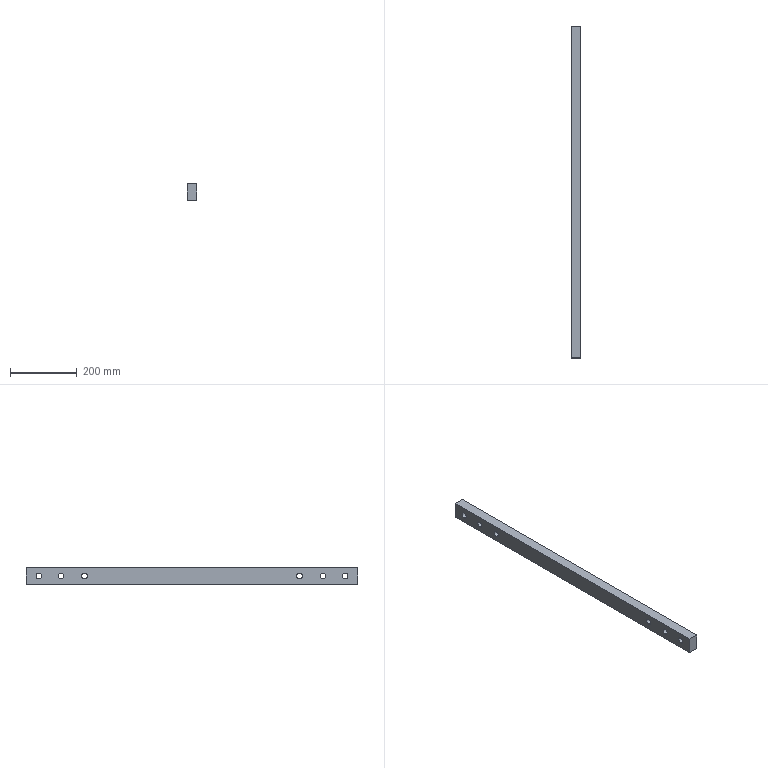Part | SolidWorks | features BaseBody 1 | 1 solid | 18 faces | box 30 x 998 x 50 mm | volume 1456144 mm3 | cylinder 12 | plane 6 | commonest cylinder face diameters 17 x12
STEP:
#1=CARTESIAN_POINT('',(15.,38.5,-8.5));
#2=VERTEX_POINT('',#1);
#3=CARTESIAN_POINT('',(15.,38.5,8.5));
#4=VERTEX_POINT('',#3);
#5=CARTESIAN_POINT('',(15.,38.5,0.));
#6=DIRECTION('',(-1.,0.,0.));
#7=DIRECTION('',(0.,0.,1.));
#8=AXIS2_PLACEMENT_3D('',#5,#6,#7);
#9=CIRCLE('',#8,8.5);
#10=EDGE_CURVE('',#2,#4,#9,.T.);
#11=ORIENTED_EDGE('',*,*,#10,.F.);
#12=CARTESIAN_POINT('',(-15.,38.5,-8.5));
#13=VERTEX_POINT('',#12);
#14=CARTESIAN_POINT('',(15.,38.5,-8.5));
#15=DIRECTION('',(-1.,0.,0.));
#16=VECTOR('',#15,1000.);
#17=LINE('',#14,#16);
#18=EDGE_CURVE('',#2,#13,#17,.T.);
#19=ORIENTED_EDGE('',*,*,#18,.T.);
#20=CARTESIAN_POINT('',(-15.,38.5,8.5));
#21=VERTEX_POINT('',#20);
#22=CARTESIAN_POINT('',(-15.,38.5,0.));
#23=DIRECTION('',(-1.,0.,0.));
#24=DIRECTION('',(0.,0.,1.));
#25=AXIS2_PLACEMENT_3D('',#22,#23,#24);
#26=CIRCLE('',#25,8.5);
#27=EDGE_CURVE('',#13,#21,#26,.T.);
#28=ORIENTED_EDGE('',*,*,#27,.T.);
#29=CARTESIAN_POINT('',(15.,38.5,8.5));
#30=DIRECTION('',(-1.,0.,0.));
#31=VECTOR('',#30,1000.);
#32=LINE('',#29,#31);
#33=EDGE_CURVE('',#4,#21,#32,.T.);
#34=ORIENTED_EDGE('',*,*,#33,.F.);
#35=EDGE_LOOP('',(#11,#19,#28,#34));
#36=FACE_OUTER_BOUND('',#35,.T.);
#37=CARTESIAN_POINT('',(15.,38.5,0.));
#38=DIRECTION('',(-1.,0.,0.));
#39=DIRECTION('',(0.,0.,1.));
#40=AXIS2_PLACEMENT_3D('',#37,#38,#39);
#41=CYLINDRICAL_SURFACE('',#40,8.5);
#42=ADVANCED_FACE('',(#36),#41,.F.);
#43=CARTESIAN_POINT('',(15.,822.359,-8.5));
#44=VERTEX_POINT('',#43);
#45=CARTESIAN_POINT('',(15.,822.359,8.5));
#46=VERTEX_POINT('',#45);
#47=CARTESIAN_POINT('',(15.,822.359,0.));
#48=DIRECTION('',(-1.,0.,0.));
#49=DIRECTION('',(0.,0.,-1.));
#50=AXIS2_PLACEMENT_3D('',#47,#48,#49);
#51=CIRCLE('',#50,8.5);
#52=EDGE_CURVE('',#44,#46,#51,.T.);
#53=ORIENTED_EDGE('',*,*,#52,.F.);
#54=CARTESIAN_POINT('',(-15.,822.359,-8.5));
#55=VERTEX_POINT('',#54);
#56=CARTESIAN_POINT('',(15.,822.359,-8.5));
#57=DIRECTION('',(-1.,0.,0.));
#58=VECTOR('',#57,1000.);
#59=LINE('',#56,#58);
#60=EDGE_CURVE('',#44,#55,#59,.T.);
#61=ORIENTED_EDGE('',*,*,#60,.T.);
#62=CARTESIAN_POINT('',(-15.,822.359,8.5));
#63=VERTEX_POINT('',#62);
#64=CARTESIAN_POINT('',(-15.,822.359,0.));
#65=DIRECTION('',(-1.,0.,0.));
#66=DIRECTION('',(0.,0.,-1.));
#67=AXIS2_PLACEMENT_3D('',#64,#65,#66);
#68=CIRCLE('',#67,8.5);
#69=EDGE_CURVE('',#55,#63,#68,.T.);
#70=ORIENTED_EDGE('',*,*,#69,.T.);
#71=CARTESIAN_POINT('',(15.,822.359,8.5));
#72=DIRECTION('',(-1.,0.,0.));
#73=VECTOR('',#72,1000.);
#74=LINE('',#71,#73);
#75=EDGE_CURVE('',#46,#63,#74,.T.);
#76=ORIENTED_EDGE('',*,*,#75,.F.);
#77=EDGE_LOOP('',(#53,#61,#70,#76));
#78=FACE_OUTER_BOUND('',#77,.T.);
#79=CARTESIAN_POINT('',(15.,822.359,0.));
#80=DIRECTION('',(-1.,0.,0.));
#81=DIRECTION('',(0.,0.,1.));
#82=AXIS2_PLACEMENT_3D('',#79,#80,#81);
#83=CYLINDRICAL_SURFACE('',#82,8.5);
#84=ADVANCED_FACE('',(#78),#83,.F.);
#85=CARTESIAN_POINT('',(15.,175.641,-8.5));
#86=VERTEX_POINT('',#85);
#87=CARTESIAN_POINT('',(15.,175.641,8.5));
#88=VERTEX_POINT('',#87);
#89=CARTESIAN_POINT('',(15.,175.641,0.));
#90=DIRECTION('',(-1.,0.,0.));
#91=DIRECTION('',(0.,0.,1.));
#92=AXIS2_PLACEMENT_3D('',#89,#90,#91);
#93=CIRCLE('',#92,8.5);
#94=EDGE_CURVE('',#86,#88,#93,.T.);
#95=ORIENTED_EDGE('',*,*,#94,.F.);
#96=CARTESIAN_POINT('',(-15.,175.641,-8.5));
#97=VERTEX_POINT('',#96);
#98=CARTESIAN_POINT('',(15.,175.641,-8.5));
#99=DIRECTION('',(-1.,0.,0.));
#100=VECTOR('',#99,1000.);
#101=LINE('',#98,#100);
#102=EDGE_CURVE('',#86,#97,#101,.T.);
#103=ORIENTED_EDGE('',*,*,#102,.T.);
#104=CARTESIAN_POINT('',(-15.,175.641,8.5));
#105=VERTEX_POINT('',#104);
#106=CARTESIAN_POINT('',(-15.,175.641,0.));
#107=DIRECTION('',(-1.,0.,0.));
#108=DIRECTION('',(0.,0.,1.));
#109=AXIS2_PLACEMENT_3D('',#106,#107,#108);
#110=CIRCLE('',#109,8.5);
#111=EDGE_CURVE('',#97,#105,#110,.T.);
#112=ORIENTED_EDGE('',*,*,#111,.T.);
#113=CARTESIAN_POINT('',(15.,175.641,8.5));
#114=DIRECTION('',(-1.,0.,0.));
#115=VECTOR('',#114,1000.);
#116=LINE('',#113,#115);
#117=EDGE_CURVE('',#88,#105,#116,.T.);
#118=ORIENTED_EDGE('',*,*,#117,.F.);
#119=EDGE_LOOP('',(#95,#103,#112,#118));
#120=FACE_OUTER_BOUND('',#119,.T.);
#121=CARTESIAN_POINT('',(15.,175.641,0.));
#122=DIRECTION('',(-1.,0.,0.));
#123=DIRECTION('',(0.,0.,1.));
#124=AXIS2_PLACEMENT_3D('',#121,#122,#123);
#125=CYLINDRICAL_SURFACE('',#124,8.5);
#126=ADVANCED_FACE('',(#120),#125,.F.);
#127=CARTESIAN_POINT('',(15.,892.899,-8.5));
#128=VERTEX_POINT('',#127);
#129=CARTESIAN_POINT('',(15.,892.899,8.5));
#130=VERTEX_POINT('',#129);
#131=CARTESIAN_POINT('',(15.,892.899,0.));
#132=DIRECTION('',(-1.,0.,0.));
#133=DIRECTION('',(0.,0.,-1.));
#134=AXIS2_PLACEMENT_3D('',#131,#132,#133);
#135=CIRCLE('',#134,8.5);
#136=EDGE_CURVE('',#128,#130,#135,.T.);
#137=ORIENTED_EDGE('',*,*,#136,.F.);
#138=CARTESIAN_POINT('',(-15.,892.899,-8.5));
#139=VERTEX_POINT('',#138);
#140=CARTESIAN_POINT('',(15.,892.899,-8.5));
#141=DIRECTION('',(-1.,0.,0.));
#142=VECTOR('',#141,1000.);
#143=LINE('',#140,#142);
#144=EDGE_CURVE('',#128,#139,#143,.T.);
#145=ORIENTED_EDGE('',*,*,#144,.T.);
#146=CARTESIAN_POINT('',(-15.,892.899,8.5));
#147=VERTEX_POINT('',#146);
#148=CARTESIAN_POINT('',(-15.,892.899,0.));
#149=DIRECTION('',(-1.,0.,0.));
#150=DIRECTION('',(0.,0.,-1.));
#151=AXIS2_PLACEMENT_3D('',#148,#149,#150);
#152=CIRCLE('',#151,8.5);
#153=EDGE_CURVE('',#139,#147,#152,.T.);
#154=ORIENTED_EDGE('',*,*,#153,.T.);
#155=CARTESIAN_POINT('',(15.,892.899,8.5));
#156=DIRECTION('',(-1.,0.,0.));
#157=VECTOR('',#156,1000.);
#158=LINE('',#155,#157);
#159=EDGE_CURVE('',#130,#147,#158,.T.);
#160=ORIENTED_EDGE('',*,*,#159,.F.);
#161=EDGE_LOOP('',(#137,#145,#154,#160));
#162=FACE_OUTER_BOUND('',#161,.T.);
#163=CARTESIAN_POINT('',(15.,892.899,0.));
#164=DIRECTION('',(-1.,0.,0.));
#165=DIRECTION('',(0.,0.,1.));
#166=AXIS2_PLACEMENT_3D('',#163,#164,#165);
#167=CYLINDRICAL_SURFACE('',#166,8.5);
#168=ADVANCED_FACE('',(#162),#167,.F.);
#169=CARTESIAN_POINT('',(15.,105.101,-8.5));
#170=VERTEX_POINT('',#169);
#171=CARTESIAN_POINT('',(15.,105.101,8.5));
#172=VERTEX_POINT('',#171);
#173=CARTESIAN_POINT('',(15.,105.101,0.));
#174=DIRECTION('',(-1.,0.,0.));
#175=DIRECTION('',(0.,0.,1.));
#176=AXIS2_PLACEMENT_3D('',#173,#174,#175);
#177=CIRCLE('',#176,8.5);
#178=EDGE_CURVE('',#170,#172,#177,.T.);
#179=ORIENTED_EDGE('',*,*,#178,.F.);
#180=CARTESIAN_POINT('',(-15.,105.101,-8.5));
#181=VERTEX_POINT('',#180);
#182=CARTESIAN_POINT('',(15.,105.101,-8.5));
#183=DIRECTION('',(-1.,0.,0.));
#184=VECTOR('',#183,1000.);
#185=LINE('',#182,#184);
#186=EDGE_CURVE('',#170,#181,#185,.T.);
#187=ORIENTED_EDGE('',*,*,#186,.T.);
#188=CARTESIAN_POINT('',(-15.,105.101,8.5));
#189=VERTEX_POINT('',#188);
#190=CARTESIAN_POINT('',(-15.,105.101,0.));
#191=DIRECTION('',(-1.,0.,0.));
#192=DIRECTION('',(0.,0.,1.));
#193=AXIS2_PLACEMENT_3D('',#190,#191,#192);
#194=CIRCLE('',#193,8.5);
#195=EDGE_CURVE('',#181,#189,#194,.T.);
#196=ORIENTED_EDGE('',*,*,#195,.T.);
#197=CARTESIAN_POINT('',(15.,105.101,8.5));
#198=DIRECTION('',(-1.,0.,0.));
#199=VECTOR('',#198,1000.);
#200=LINE('',#197,#199);
#201=EDGE_CURVE('',#172,#189,#200,.T.);
#202=ORIENTED_EDGE('',*,*,#201,.F.);
#203=EDGE_LOOP('',(#179,#187,#196,#202));
#204=FACE_OUTER_BOUND('',#203,.T.);
#205=CARTESIAN_POINT('',(15.,105.101,0.));
#206=DIRECTION('',(-1.,0.,0.));
#207=DIRECTION('',(0.,0.,1.));
#208=AXIS2_PLACEMENT_3D('',#205,#206,#207);
#209=CYLINDRICAL_SURFACE('',#208,8.5);
#210=ADVANCED_FACE('',(#204),#209,.F.);
#211=CARTESIAN_POINT('',(15.,959.5,-8.5));
#212=VERTEX_POINT('',#211);
#213=CARTESIAN_POINT('',(15.,959.5,8.5));
#214=VERTEX_POINT('',#213);
#215=CARTESIAN_POINT('',(15.,959.5,0.));
#216=DIRECTION('',(-1.,0.,0.));
#217=DIRECTION('',(0.,0.,-1.));
#218=AXIS2_PLACEMENT_3D('',#215,#216,#217);
#219=CIRCLE('',#218,8.5);
#220=EDGE_CURVE('',#212,#214,#219,.T.);
#221=ORIENTED_EDGE('',*,*,#220,.F.);
#222=CARTESIAN_POINT('',(-15.,959.5,-8.5));
#223=VERTEX_POINT('',#222);
#224=CARTESIAN_POINT('',(15.,959.5,-8.5));
#225=DIRECTION('',(-1.,0.,0.));
#226=VECTOR('',#225,1000.);
#227=LINE('',#224,#226);
#228=EDGE_CURVE('',#212,#223,#227,.T.);
#229=ORIENTED_EDGE('',*,*,#228,.T.);
#230=CARTESIAN_POINT('',(-15.,959.5,8.5));
#231=VERTEX_POINT('',#230);
#232=CARTESIAN_POINT('',(-15.,959.5,0.));
#233=DIRECTION('',(-1.,0.,0.));
#234=DIRECTION('',(0.,0.,-1.));
#235=AXIS2_PLACEMENT_3D('',#232,#233,#234);
#236=CIRCLE('',#235,8.5);
#237=EDGE_CURVE('',#223,#231,#236,.T.);
#238=ORIENTED_EDGE('',*,*,#237,.T.);
#239=CARTESIAN_POINT('',(15.,959.5,8.5));
#240=DIRECTION('',(-1.,0.,0.));
#241=VECTOR('',#240,1000.);
#242=LINE('',#239,#241);
#243=EDGE_CURVE('',#214,#231,#242,.T.);
#244=ORIENTED_EDGE('',*,*,#243,.F.);
#245=EDGE_LOOP('',(#221,#229,#238,#244));
#246=FACE_OUTER_BOUND('',#245,.T.);
#247=CARTESIAN_POINT('',(15.,959.5,0.));
#248=DIRECTION('',(-1.,0.,0.));
#249=DIRECTION('',(0.,0.,1.));
#250=AXIS2_PLACEMENT_3D('',#247,#248,#249);
#251=CYLINDRICAL_SURFACE('',#250,8.5);
#252=ADVANCED_FACE('',(#246),#251,.F.);
#253=CARTESIAN_POINT('',(15.,38.5,0.));
#254=DIRECTION('',(-1.,0.,0.));
#255=DIRECTION('',(0.,0.,1.));
#256=AXIS2_PLACEMENT_3D('',#253,#254,#255);
#257=CIRCLE('',#256,8.5);
#258=EDGE_CURVE('',#4,#2,#257,.T.);
#259=ORIENTED_EDGE('',*,*,#258,.T.);
#260=ORIENTED_EDGE('',*,*,#10,.T.);
#261=EDGE_LOOP('',(#259,#260));
#262=FACE_BOUND('',#261,.T.);
#263=CARTESIAN_POINT('',(15.,822.359,0.));
#264=DIRECTION('',(-1.,0.,0.));
#265=DIRECTION('',(0.,0.,-1.));
#266=AXIS2_PLACEMENT_3D('',#263,#264,#265);
#267=CIRCLE('',#266,8.5);
#268=EDGE_CURVE('',#46,#44,#267,.T.);
#269=ORIENTED_EDGE('',*,*,#268,.T.);
#270=ORIENTED_EDGE('',*,*,#52,.T.);
#271=EDGE_LOOP('',(#269,#270));
#272=FACE_BOUND('',#271,.T.);
#273=CARTESIAN_POINT('',(15.,175.641,0.));
#274=DIRECTION('',(-1.,0.,0.));
#275=DIRECTION('',(0.,0.,1.));
#276=AXIS2_PLACEMENT_3D('',#273,#274,#275);
#277=CIRCLE('',#276,8.5);
#278=EDGE_CURVE('',#88,#86,#277,.T.);
#279=ORIENTED_EDGE('',*,*,#278,.T.);
#280=ORIENTED_EDGE('',*,*,#94,.T.);
#281=EDGE_LOOP('',(#279,#280));
#282=FACE_BOUND('',#281,.T.);
#283=CARTESIAN_POINT('',(15.,892.899,0.));
#284=DIRECTION('',(-1.,0.,0.));
#285=DIRECTION('',(0.,0.,-1.));
#286=AXIS2_PLACEMENT_3D('',#283,#284,#285);
#287=CIRCLE('',#286,8.5);
#288=EDGE_CURVE('',#130,#128,#287,.T.);
#289=ORIENTED_EDGE('',*,*,#288,.T.);
#290=ORIENTED_EDGE('',*,*,#136,.T.);
#291=EDGE_LOOP('',(#289,#290));
#292=FACE_BOUND('',#291,.T.);
#293=CARTESIAN_POINT('',(15.,105.101,0.));
#294=DIRECTION('',(-1.,0.,0.));
#295=DIRECTION('',(0.,0.,1.));
#296=AXIS2_PLACEMENT_3D('',#293,#294,#295);
#297=CIRCLE('',#296,8.5);
#298=EDGE_CURVE('',#172,#170,#297,.T.);
#299=ORIENTED_EDGE('',*,*,#298,.T.);
#300=ORIENTED_EDGE('',*,*,#178,.T.);
#301=EDGE_LOOP('',(#299,#300));
#302=FACE_BOUND('',#301,.T.);
#303=CARTESIAN_POINT('',(15.,959.5,0.));
#304=DIRECTION('',(-1.,0.,0.));
#305=DIRECTION('',(0.,0.,-1.));
#306=AXIS2_PLACEMENT_3D('',#303,#304,#305);
#307=CIRCLE('',#306,8.5);
#308=EDGE_CURVE('',#214,#212,#307,.T.);
#309=ORIENTED_EDGE('',*,*,#308,.T.);
#310=ORIENTED_EDGE('',*,*,#220,.T.);
#311=EDGE_LOOP('',(#309,#310));
#312=FACE_BOUND('',#311,.T.);
#313=CARTESIAN_POINT('',(15.,0.,25.));
#314=VERTEX_POINT('',#313);
#315=CARTESIAN_POINT('',(15.,0.,-25.));
#316=VERTEX_POINT('',#315);
#317=CARTESIAN_POINT('',(15.,0.,-25.));
#318=DIRECTION('',(0.,0.,-1.));
#319=VECTOR('',#318,1000.);
#320=LINE('',#317,#319);
#321=EDGE_CURVE('',#314,#316,#320,.T.);
#322=ORIENTED_EDGE('',*,*,#321,.T.);
#323=CARTESIAN_POINT('',(15.,998.,-25.));
#324=VERTEX_POINT('',#323);
#325=CARTESIAN_POINT('',(15.,998.,-25.));
#326=DIRECTION('',(0.,-1.,0.));
#327=VECTOR('',#326,1000.);
#328=LINE('',#325,#327);
#329=EDGE_CURVE('',#324,#316,#328,.T.);
#330=ORIENTED_EDGE('',*,*,#329,.F.);
#331=CARTESIAN_POINT('',(15.,998.,25.));
#332=VERTEX_POINT('',#331);
#333=CARTESIAN_POINT('',(15.,998.,-25.));
#334=DIRECTION('',(0.,0.,-1.));
#335=VECTOR('',#334,1000.);
#336=LINE('',#333,#335);
#337=EDGE_CURVE('',#332,#324,#336,.T.);
#338=ORIENTED_EDGE('',*,*,#337,.F.);
#339=CARTESIAN_POINT('',(15.,998.,25.));
#340=DIRECTION('',(0.,-1.,0.));
#341=VECTOR('',#340,1000.);
#342=LINE('',#339,#341);
#343=EDGE_CURVE('',#332,#314,#342,.T.);
#344=ORIENTED_EDGE('',*,*,#343,.T.);
#345=EDGE_LOOP('',(#322,#330,#338,#344));
#346=FACE_OUTER_BOUND('',#345,.T.);
#347=CARTESIAN_POINT('',(15.,998.,-25.));
#348=DIRECTION('',(-1.,0.,0.));
#349=DIRECTION('',(0.,0.,1.));
#350=AXIS2_PLACEMENT_3D('',#347,#348,#349);
#351=PLANE('',#350);
#352=ADVANCED_FACE('',(#262,#272,#282,#292,#302,#312,#346),#351,.F.);
#353=CARTESIAN_POINT('',(-15.,0.,-25.));
#354=VERTEX_POINT('',#353);
#355=CARTESIAN_POINT('',(-15.,0.,-25.));
#356=DIRECTION('',(-1.,0.,0.));
#357=VECTOR('',#356,1000.);
#358=LINE('',#355,#357);
#359=EDGE_CURVE('',#316,#354,#358,.T.);
#360=ORIENTED_EDGE('',*,*,#359,.T.);
#361=CARTESIAN_POINT('',(-15.,998.,-25.));
#362=VERTEX_POINT('',#361);
#363=CARTESIAN_POINT('',(-15.,998.,-25.));
#364=DIRECTION('',(0.,-1.,0.));
#365=VECTOR('',#364,1000.);
#366=LINE('',#363,#365);
#367=EDGE_CURVE('',#362,#354,#366,.T.);
#368=ORIENTED_EDGE('',*,*,#367,.F.);
#369=CARTESIAN_POINT('',(-15.,998.,-25.));
#370=DIRECTION('',(-1.,0.,0.));
#371=VECTOR('',#370,1000.);
#372=LINE('',#369,#371);
#373=EDGE_CURVE('',#324,#362,#372,.T.);
#374=ORIENTED_EDGE('',*,*,#373,.F.);
#375=ORIENTED_EDGE('',*,*,#329,.T.);
#376=EDGE_LOOP('',(#360,#368,#374,#375));
#377=FACE_OUTER_BOUND('',#376,.T.);
#378=CARTESIAN_POINT('',(-15.,998.,-25.));
#379=DIRECTION('',(0.,0.,1.));
#380=DIRECTION('',(1.,0.,0.));
#381=AXIS2_PLACEMENT_3D('',#378,#379,#380);
#382=PLANE('',#381);
#383=ADVANCED_FACE('',(#377),#382,.F.);
#384=CARTESIAN_POINT('',(-15.,38.5,0.));
#385=DIRECTION('',(-1.,0.,0.));
#386=DIRECTION('',(0.,0.,1.));
#387=AXIS2_PLACEMENT_3D('',#384,#385,#386);
#388=CIRCLE('',#387,8.5);
#389=EDGE_CURVE('',#21,#13,#388,.T.);
#390=ORIENTED_EDGE('',*,*,#389,.F.);
#391=ORIENTED_EDGE('',*,*,#27,.F.);
#392=EDGE_LOOP('',(#390,#391));
#393=FACE_BOUND('',#392,.T.);
#394=CARTESIAN_POINT('',(-15.,822.359,0.));
#395=DIRECTION('',(-1.,0.,0.));
#396=DIRECTION('',(0.,0.,-1.));
#397=AXIS2_PLACEMENT_3D('',#394,#395,#396);
#398=CIRCLE('',#397,8.5);
#399=EDGE_CURVE('',#63,#55,#398,.T.);
#400=ORIENTED_EDGE('',*,*,#399,.F.);
#401=ORIENTED_EDGE('',*,*,#69,.F.);
#402=EDGE_LOOP('',(#400,#401));
#403=FACE_BOUND('',#402,.T.);
#404=CARTESIAN_POINT('',(-15.,175.641,0.));
#405=DIRECTION('',(-1.,0.,0.));
#406=DIRECTION('',(0.,0.,1.));
#407=AXIS2_PLACEMENT_3D('',#404,#405,#406);
#408=CIRCLE('',#407,8.5);
#409=EDGE_CURVE('',#105,#97,#408,.T.);
#410=ORIENTED_EDGE('',*,*,#409,.F.);
#411=ORIENTED_EDGE('',*,*,#111,.F.);
#412=EDGE_LOOP('',(#410,#411));
#413=FACE_BOUND('',#412,.T.);
#414=CARTESIAN_POINT('',(-15.,892.899,0.));
#415=DIRECTION('',(-1.,0.,0.));
#416=DIRECTION('',(0.,0.,-1.));
#417=AXIS2_PLACEMENT_3D('',#414,#415,#416);
#418=CIRCLE('',#417,8.5);
#419=EDGE_CURVE('',#147,#139,#418,.T.);
#420=ORIENTED_EDGE('',*,*,#419,.F.);
#421=ORIENTED_EDGE('',*,*,#153,.F.);
#422=EDGE_LOOP('',(#420,#421));
#423=FACE_BOUND('',#422,.T.);
#424=CARTESIAN_POINT('',(-15.,105.101,0.));
#425=DIRECTION('',(-1.,0.,0.));
#426=DIRECTION('',(0.,0.,1.));
#427=AXIS2_PLACEMENT_3D('',#424,#425,#426);
#428=CIRCLE('',#427,8.5);
#429=EDGE_CURVE('',#189,#181,#428,.T.);
#430=ORIENTED_EDGE('',*,*,#429,.F.);
#431=ORIENTED_EDGE('',*,*,#195,.F.);
#432=EDGE_LOOP('',(#430,#431));
#433=FACE_BOUND('',#432,.T.);
#434=CARTESIAN_POINT('',(-15.,959.5,0.));
#435=DIRECTION('',(-1.,0.,0.));
#436=DIRECTION('',(0.,0.,-1.));
#437=AXIS2_PLACEMENT_3D('',#434,#435,#436);
#438=CIRCLE('',#437,8.5);
#439=EDGE_CURVE('',#231,#223,#438,.T.);
#440=ORIENTED_EDGE('',*,*,#439,.F.);
#441=ORIENTED_EDGE('',*,*,#237,.F.);
#442=EDGE_LOOP('',(#440,#441));
#443=FACE_BOUND('',#442,.T.);
#444=CARTESIAN_POINT('',(-15.,0.,25.));
#445=VERTEX_POINT('',#444);
#446=CARTESIAN_POINT('',(-15.,0.,-25.));
#447=DIRECTION('',(0.,0.,1.));
#448=VECTOR('',#447,1000.);
#449=LINE('',#446,#448);
#450=EDGE_CURVE('',#354,#445,#449,.T.);
#451=ORIENTED_EDGE('',*,*,#450,.T.);
#452=CARTESIAN_POINT('',(-15.,998.,25.));
#453=VERTEX_POINT('',#452);
#454=CARTESIAN_POINT('',(-15.,998.,25.));
#455=DIRECTION('',(0.,-1.,0.));
#456=VECTOR('',#455,1000.);
#457=LINE('',#454,#456);
#458=EDGE_CURVE('',#453,#445,#457,.T.);
#459=ORIENTED_EDGE('',*,*,#458,.F.);
#460=CARTESIAN_POINT('',(-15.,998.,-25.));
#461=DIRECTION('',(0.,0.,1.));
#462=VECTOR('',#461,1000.);
#463=LINE('',#460,#462);
#464=EDGE_CURVE('',#362,#453,#463,.T.);
#465=ORIENTED_EDGE('',*,*,#464,.F.);
#466=ORIENTED_EDGE('',*,*,#367,.T.);
#467=EDGE_LOOP('',(#451,#459,#465,#466));
#468=FACE_OUTER_BOUND('',#467,.T.);
#469=CARTESIAN_POINT('',(-15.,998.,-25.));
#470=DIRECTION('',(1.,0.,0.));
#471=DIRECTION('',(0.,0.,-1.));
#472=AXIS2_PLACEMENT_3D('',#469,#470,#471);
#473=PLANE('',#472);
#474=ADVANCED_FACE('',(#393,#403,#413,#423,#433,#443,#468),#473,.F.);
#475=CARTESIAN_POINT('',(-15.,0.,25.));
#476=DIRECTION('',(1.,0.,0.));
#477=VECTOR('',#476,1000.);
#478=LINE('',#475,#477);
#479=EDGE_CURVE('',#445,#314,#478,.T.);
#480=ORIENTED_EDGE('',*,*,#479,.T.);
#481=ORIENTED_EDGE('',*,*,#343,.F.);
#482=CARTESIAN_POINT('',(-15.,998.,25.));
#483=DIRECTION('',(1.,0.,0.));
#484=VECTOR('',#483,1000.);
#485=LINE('',#482,#484);
#486=EDGE_CURVE('',#453,#332,#485,.T.);
#487=ORIENTED_EDGE('',*,*,#486,.F.);
#488=ORIENTED_EDGE('',*,*,#458,.T.);
#489=EDGE_LOOP('',(#480,#481,#487,#488));
#490=FACE_OUTER_BOUND('',#489,.T.);
#491=CARTESIAN_POINT('',(-15.,998.,25.));
#492=DIRECTION('',(0.,0.,-1.));
#493=DIRECTION('',(-1.,0.,0.));
#494=AXIS2_PLACEMENT_3D('',#491,#492,#493);
#495=PLANE('',#494);
#496=ADVANCED_FACE('',(#490),#495,.F.);
#497=ORIENTED_EDGE('',*,*,#337,.T.);
#498=ORIENTED_EDGE('',*,*,#373,.T.);
#499=ORIENTED_EDGE('',*,*,#464,.T.);
#500=ORIENTED_EDGE('',*,*,#486,.T.);
#501=EDGE_LOOP('',(#497,#498,#499,#500));
#502=FACE_OUTER_BOUND('',#501,.T.);
#503=CARTESIAN_POINT('',(0.,998.,0.));
#504=DIRECTION('',(0.,1.,0.));
#505=DIRECTION('',(0.,0.,1.));
#506=AXIS2_PLACEMENT_3D('',#503,#504,#505);
#507=PLANE('',#506);
#508=ADVANCED_FACE('',(#502),#507,.T.);
#509=ORIENTED_EDGE('',*,*,#321,.F.);
#510=ORIENTED_EDGE('',*,*,#479,.F.);
#511=ORIENTED_EDGE('',*,*,#450,.F.);
#512=ORIENTED_EDGE('',*,*,#359,.F.);
#513=EDGE_LOOP('',(#509,#510,#511,#512));
#514=FACE_OUTER_BOUND('',#513,.T.);
#515=CARTESIAN_POINT('',(0.,0.,0.));
#516=DIRECTION('',(0.,1.,0.));
#517=DIRECTION('',(0.,0.,1.));
#518=AXIS2_PLACEMENT_3D('',#515,#516,#517);
#519=PLANE('',#518);
#520=ADVANCED_FACE('',(#514),#519,.F.);
#521=ORIENTED_EDGE('',*,*,#228,.F.);
#522=ORIENTED_EDGE('',*,*,#308,.F.);
#523=ORIENTED_EDGE('',*,*,#243,.T.);
#524=ORIENTED_EDGE('',*,*,#439,.T.);
#525=EDGE_LOOP('',(#521,#522,#523,#524));
#526=FACE_OUTER_BOUND('',#525,.T.);
#527=CARTESIAN_POINT('',(15.,959.5,0.));
#528=DIRECTION('',(-1.,0.,0.));
#529=DIRECTION('',(0.,0.,1.));
#530=AXIS2_PLACEMENT_3D('',#527,#528,#529);
#531=CYLINDRICAL_SURFACE('',#530,8.5);
#532=ADVANCED_FACE('',(#526),#531,.F.);
#533=ORIENTED_EDGE('',*,*,#186,.F.);
#534=ORIENTED_EDGE('',*,*,#298,.F.);
#535=ORIENTED_EDGE('',*,*,#201,.T.);
#536=ORIENTED_EDGE('',*,*,#429,.T.);
#537=EDGE_LOOP('',(#533,#534,#535,#536));
#538=FACE_OUTER_BOUND('',#537,.T.);
#539=CARTESIAN_POINT('',(15.,105.101,0.));
#540=DIRECTION('',(-1.,0.,0.));
#541=DIRECTION('',(0.,0.,1.));
#542=AXIS2_PLACEMENT_3D('',#539,#540,#541);
#543=CYLINDRICAL_SURFACE('',#542,8.5);
#544=ADVANCED_FACE('',(#538),#543,.F.);
#545=ORIENTED_EDGE('',*,*,#144,.F.);
#546=ORIENTED_EDGE('',*,*,#288,.F.);
#547=ORIENTED_EDGE('',*,*,#159,.T.);
#548=ORIENTED_EDGE('',*,*,#419,.T.);
#549=EDGE_LOOP('',(#545,#546,#547,#548));
#550=FACE_OUTER_BOUND('',#549,.T.);
#551=CARTESIAN_POINT('',(15.,892.899,0.));
#552=DIRECTION('',(-1.,0.,0.));
#553=DIRECTION('',(0.,0.,1.));
#554=AXIS2_PLACEMENT_3D('',#551,#552,#553);
#555=CYLINDRICAL_SURFACE('',#554,8.5);
#556=ADVANCED_FACE('',(#550),#555,.F.);
#557=ORIENTED_EDGE('',*,*,#102,.F.);
#558=ORIENTED_EDGE('',*,*,#278,.F.);
#559=ORIENTED_EDGE('',*,*,#117,.T.);
#560=ORIENTED_EDGE('',*,*,#409,.T.);
#561=EDGE_LOOP('',(#557,#558,#559,#560));
#562=FACE_OUTER_BOUND('',#561,.T.);
#563=CARTESIAN_POINT('',(15.,175.641,0.));
#564=DIRECTION('',(-1.,0.,0.));
#565=DIRECTION('',(0.,0.,1.));
#566=AXIS2_PLACEMENT_3D('',#563,#564,#565);
#567=CYLINDRICAL_SURFACE('',#566,8.5);
#568=ADVANCED_FACE('',(#562),#567,.F.);
#569=ORIENTED_EDGE('',*,*,#60,.F.);
#570=ORIENTED_EDGE('',*,*,#268,.F.);
#571=ORIENTED_EDGE('',*,*,#75,.T.);
#572=ORIENTED_EDGE('',*,*,#399,.T.);
#573=EDGE_LOOP('',(#569,#570,#571,#572));
#574=FACE_OUTER_BOUND('',#573,.T.);
#575=CARTESIAN_POINT('',(15.,822.359,0.));
#576=DIRECTION('',(-1.,0.,0.));
#577=DIRECTION('',(0.,0.,1.));
#578=AXIS2_PLACEMENT_3D('',#575,#576,#577);
#579=CYLINDRICAL_SURFACE('',#578,8.5);
#580=ADVANCED_FACE('',(#574),#579,.F.);
#581=ORIENTED_EDGE('',*,*,#18,.F.);
#582=ORIENTED_EDGE('',*,*,#258,.F.);
#583=ORIENTED_EDGE('',*,*,#33,.T.);
#584=ORIENTED_EDGE('',*,*,#389,.T.);
#585=EDGE_LOOP('',(#581,#582,#583,#584));
#586=FACE_OUTER_BOUND('',#585,.T.);
#587=CARTESIAN_POINT('',(15.,38.5,0.));
#588=DIRECTION('',(-1.,0.,0.));
#589=DIRECTION('',(0.,0.,1.));
#590=AXIS2_PLACEMENT_3D('',#587,#588,#589);
#591=CYLINDRICAL_SURFACE('',#590,8.5);
#592=ADVANCED_FACE('',(#586),#591,.F.);
#593=CLOSED_SHELL('',(#42,#84,#126,#168,#210,#252,#352,#383,#474,#496,#508,#520,#532,#544,#556,#568,#580,#592));
#594=MANIFOLD_SOLID_BREP('',#593);
#595=CARTESIAN_POINT('',(0.,0.,0.));
#596=DIRECTION('',(0.,0.,1.));
#597=DIRECTION('',(1.,0.,0.));
#598=AXIS2_PLACEMENT_3D('',#595,#596,#597);
#599=(LENGTH_UNIT()NAMED_UNIT(*)SI_UNIT(.MILLI.,.METRE.));
#600=UNCERTAINTY_MEASURE_WITH_UNIT(LENGTH_MEASURE(0.00001),#599,'','');
#601=(NAMED_UNIT(*)PLANE_ANGLE_UNIT()SI_UNIT($,.RADIAN.));
#602=(NAMED_UNIT(*)SI_UNIT($,.STERADIAN.)SOLID_ANGLE_UNIT());
#603=(GEOMETRIC_REPRESENTATION_CONTEXT(3)GLOBAL_UNCERTAINTY_ASSIGNED_CONTEXT((#600))GLOBAL_UNIT_ASSIGNED_CONTEXT((#599,#601,#602))REPRESENTATION_CONTEXT('',''));
#604=ADVANCED_BREP_SHAPE_REPRESENTATION('',(#594,#598),#603);